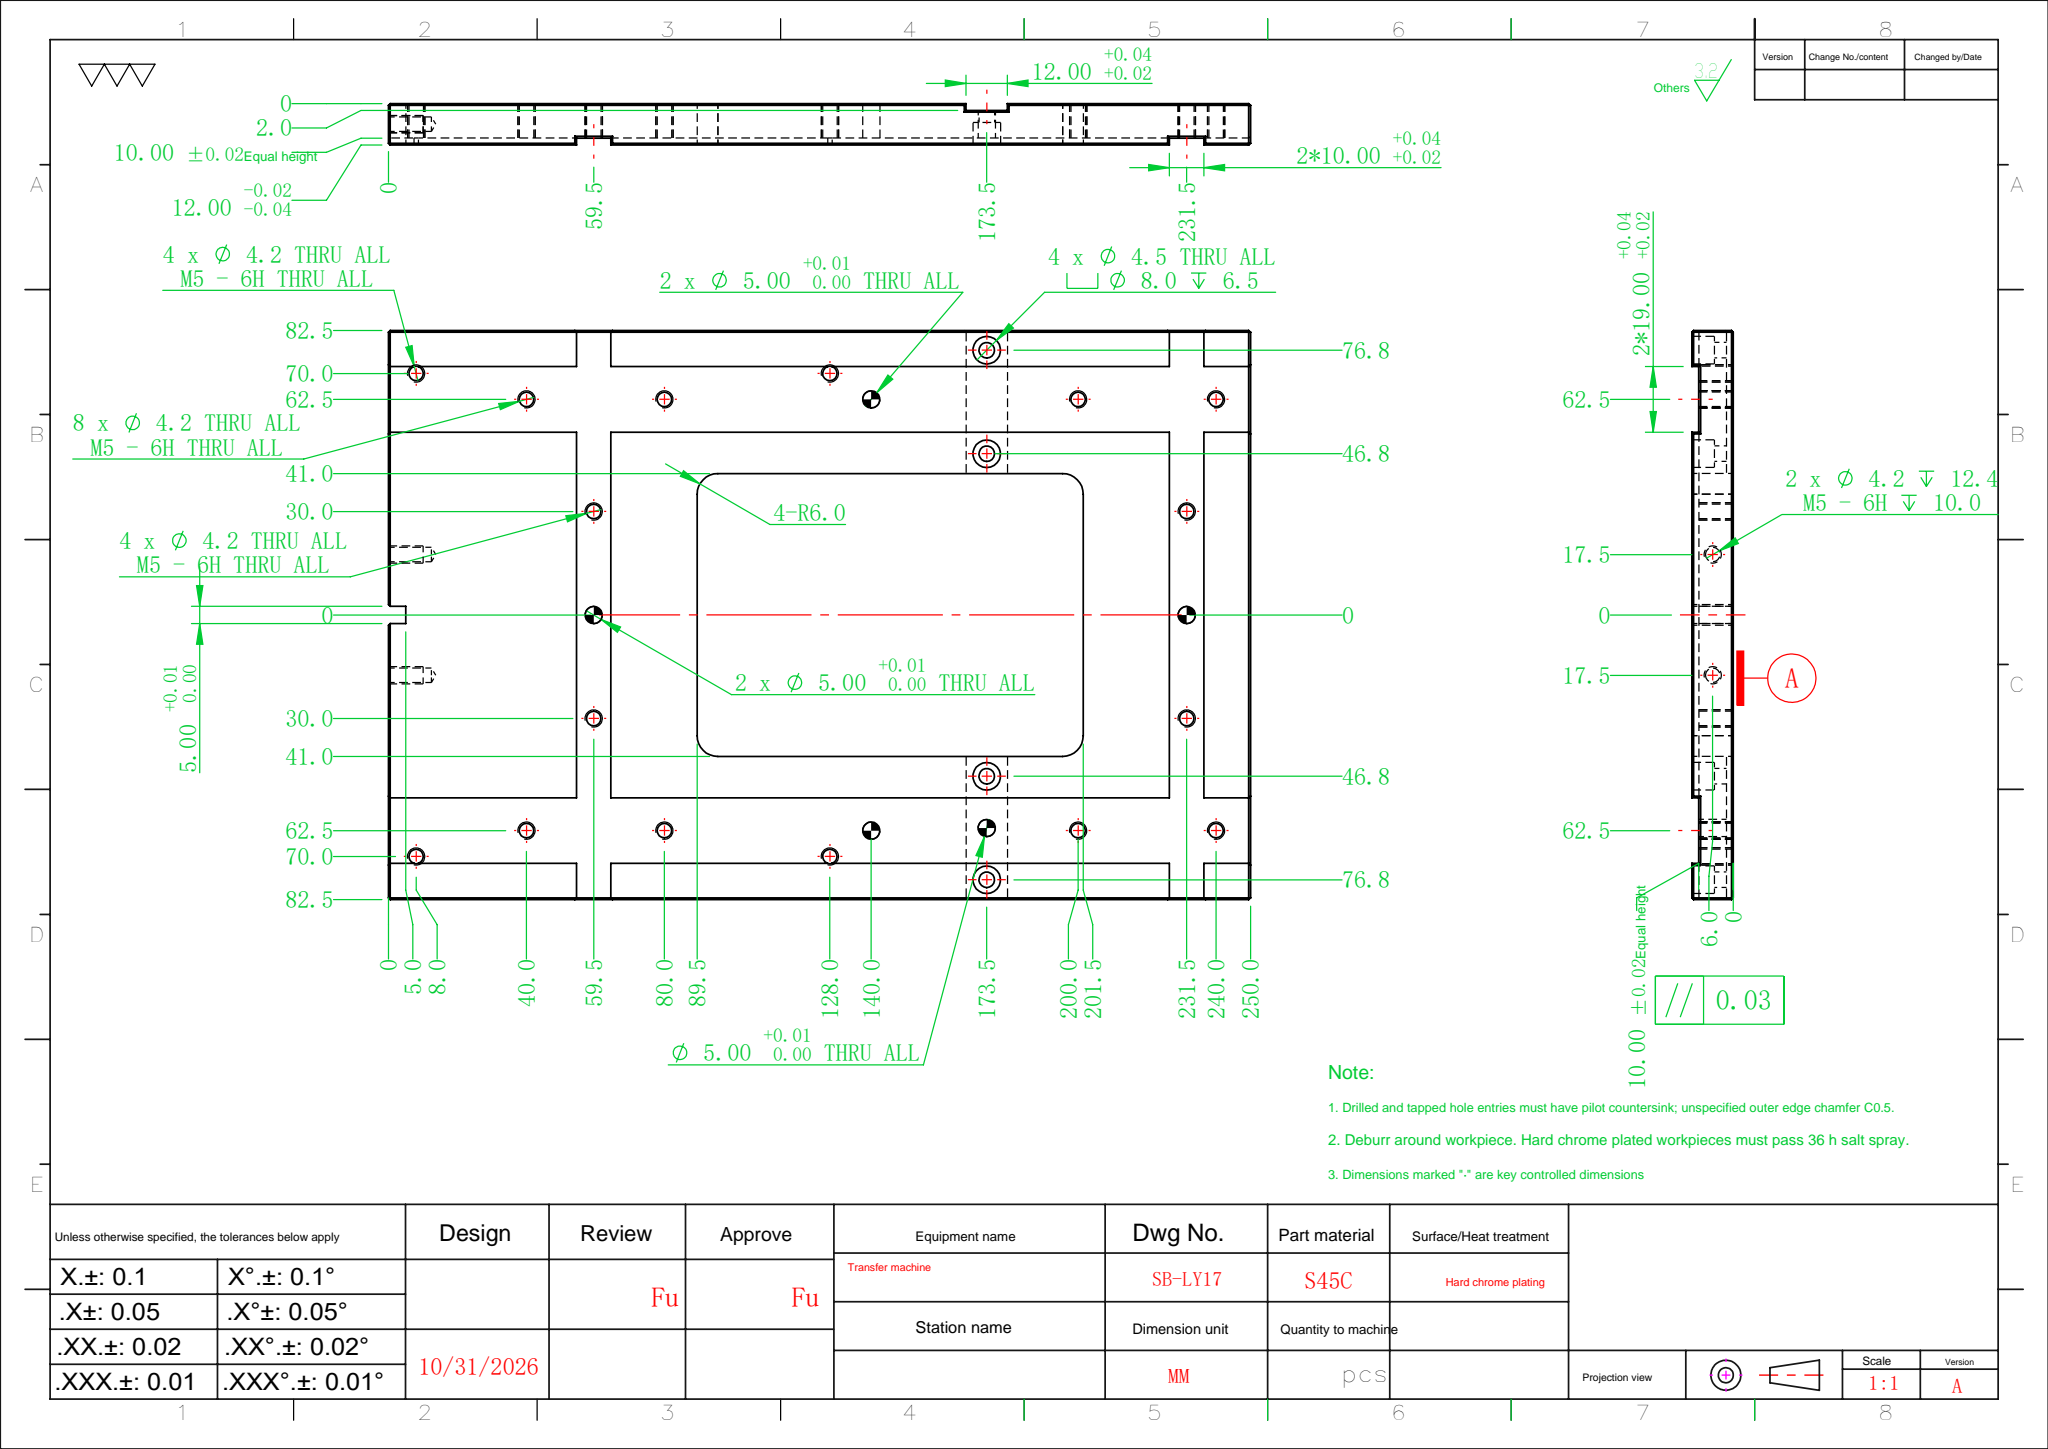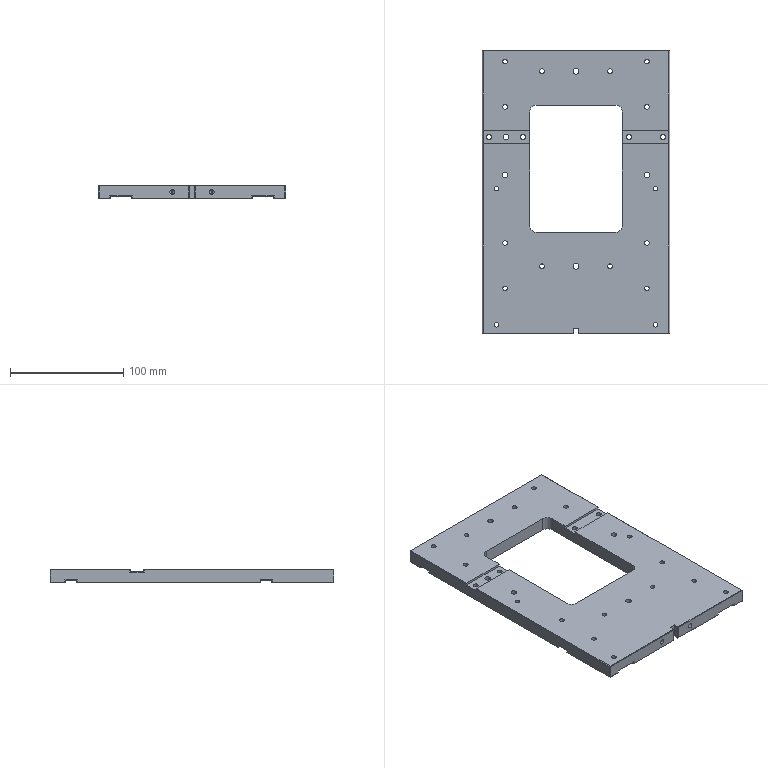Part | SolidWorks | features HoleWzd 8, Cut 5, ICE 2, Chamfer 1, Extrusion 1 | 1 solid | 196 faces | box 165 x 250 x 12 mm | volume 353527 mm3 | plane 126 | cylinder 66 | cone 4 | commonest cylinder face diameters 4.2 x36 5 x10 4.5 x8 8 x8 12 x4